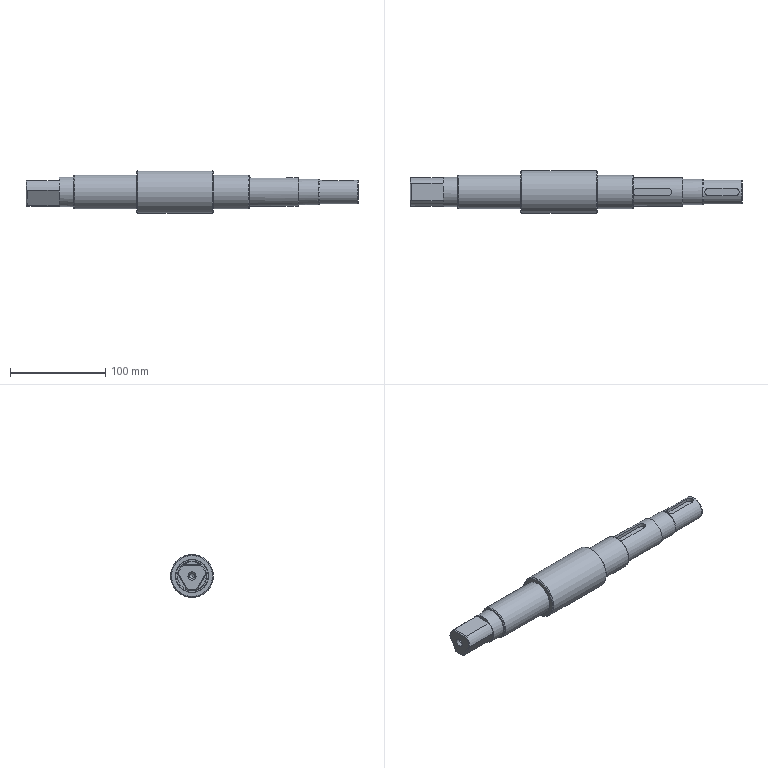NC program | NX | posted with a generic post | part box 348.4 x 45 x 45 mm
Whole program:
N10 G17 G21 G94 G90
(刀补6 , TOOL : D6)
N12 T06 M6
N14 G54
N16 G17 G0 G90 X94.077 Y-0.933 B0. C0. S4500 M3
N18 G43 Z30. H6
N20 Z-4.466
N22 G94 G1 X96.205 Z-4.578 F1000.
N24 X96.342 Y-0.932 Z-4.585
N26 X96.626 Y-0.84 Z-4.601
N28 X96.867 Y-0.664 Z-4.616
N30 X97.041 Y-0.422 Z-4.632
N32 X97.13 Y-0.137 Z-4.648
N34 Y0.137 Z-4.662
N36 X97.041 Y0.421 Z-4.678
N38 X96.867 Y0.664 Z-4.693
N40 X96.626 Y0.839 Z-4.709
N42 X96.342 Y0.931 Z-4.724
N44 X96.201 Y0.933 Z-4.732
N46 X80.298 Z-5.565
N48 G41 X80.2 Y0.95 D6
N50 X64.195 F1650.
N52 G3 X63.253 Y0. R0.95
N54 X64.195 Y-0.95 R0.95
N56 G1 X96.205
N58 G3 X97.148 Y0. R0.95
N60 X96.205 Y0.95 R0.95
N62 G1 X80.2
N64 X74.533 Z-5.664
N66 X64.195
N68 G3 X63.253 Y0. R0.95
N70 X64.195 Y-0.95 R0.95
N72 G1 X96.205
N74 G3 X97.148 Y0. R0.95
N76 X96.205 Y0.95 R0.95
N78 G1 X80.2
N80 X74.533 Z-5.763
N82 X64.195
N84 G3 X63.253 Y0. R0.95
N86 X64.195 Y-0.95 R0.95
N88 G1 X96.205
N90 G3 X97.148 Y0. R0.95
N92 X96.205 Y0.95 R0.95
N94 G1 X80.2
N96 X74.533 Z-5.862
N98 X64.195
N100 G3 X63.253 Y0. R0.95
N102 X64.195 Y-0.95 R0.95
N104 G1 X96.205
N106 G3 X97.148 Y0. R0.95
N108 X96.205 Y0.95 R0.95
N110 G1 X80.2
N112 X74.533 Z-5.961
N114 X64.195
N116 G3 X63.253 Y0. R0.95
N118 X64.195 Y-0.95 R0.95
N120 G1 X96.205
N122 G3 X97.148 Y0. R0.95
N124 X96.205 Y0.95 R0.95
N126 G1 X80.2
N128 X74.533 Z-6.06
N130 X64.195
N132 G3 X63.253 Y0. R0.95
N134 X64.195 Y-0.95 R0.95
N136 G1 X96.205
N138 G3 X97.148 Y0. R0.95
N140 X96.205 Y0.95 R0.95
N142 G1 X80.2
N144 X74.533 Z-6.159
N146 X64.195
N148 G3 X63.253 Y0. R0.95
N150 X64.195 Y-0.95 R0.95
N152 G1 X96.205
N154 G3 X97.148 Y0. R0.95
N156 X96.205 Y0.95 R0.95
N158 G1 X80.2
N160 X74.533 Z-6.258
N162 X64.195
N164 G3 X63.253 Y0. R0.95
N166 X64.195 Y-0.95 R0.95
N168 G1 X96.205
N170 G3 X97.148 Y0. R0.95
N172 X96.205 Y0.95 R0.95
N174 G1 X80.2
N176 X74.533 Z-6.357
N178 X64.195
N180 G3 X63.253 Y0. R0.95
N182 X64.195 Y-0.95 R0.95
N184 G1 X96.205
N186 G3 X97.148 Y0. R0.95
N188 X96.205 Y0.95 R0.95
N190 G1 X80.2
N192 X74.533 Z-6.455
N194 X64.195
N196 G3 X63.253 Y0. R0.95
N198 X64.195 Y-0.95 R0.95
N200 G1 X96.205
N202 G3 X97.148 Y0. R0.95
N204 X96.205 Y0.95 R0.95
N206 G1 X80.2
N208 X74.533 Z-6.554
N210 X64.195
N212 G3 X63.253 Y0. R0.95
N214 X64.195 Y-0.95 R0.95
N216 G1 X96.205
N218 G3 X97.148 Y0. R0.95
N220 X96.205 Y0.95 R0.95
N222 G1 X80.2
N224 X74.533 Z-6.653
N226 X64.195
N228 G3 X63.253 Y0. R0.95
N230 X64.195 Y-0.95 R0.95
N232 G1 X96.205
N234 G3 X97.148 Y0. R0.95
N236 X96.205 Y0.95 R0.95
N238 G1 X80.2
N240 X74.533 Z-6.752
N242 X64.195
N244 G3 X63.253 Y0. R0.95
N246 X64.195 Y-0.95 R0.95
N248 G1 X96.205
N250 G3 X97.148 Y0. R0.95
N252 X96.205 Y0.95 R0.95
N254 G1 X80.2
N256 X74.533 Z-6.851
N258 X64.195
N260 G3 X63.253 Y0. R0.95
N262 X64.195 Y-0.95 R0.95
N264 G1 X96.205
N266 G3 X97.148 Y0. R0.95
N268 X96.205 Y0.95 R0.95
N270 G1 X80.2
N272 X74.533 Z-6.95
N274 X64.195
N276 G3 X63.253 Y0. R0.95
N278 X64.195 Y-0.95 R0.95
N280 G1 X96.205
N282 G3 X97.148 Y0. R0.95
N284 X96.205 Y0.95 R0.95
N286 G1 X80.2
N288 X74.533 Z-7.049
N290 X64.195
N292 G3 X63.253 Y0. R0.95
N294 X64.195 Y-0.95 R0.95
N296 G1 X96.205
N298 G3 X97.148 Y0. R0.95
N300 X96.205 Y0.95 R0.95
N302 G1 X80.2
N304 X74.533 Z-7.148
N306 X64.195
N308 G3 X63.253 Y0. R0.95
N310 X64.195 Y-0.95 R0.95
N312 G1 X96.205
N314 G3 X97.148 Y0. R0.95
N316 X96.205 Y0.95 R0.95
N318 G1 X80.2
N320 X74.533 Z-7.247
N322 X64.195
N324 G3 X63.253 Y0. R0.95
N326 X64.195 Y-0.95 R0.95
N328 G1 X96.205
N330 G3 X97.148 Y0. R0.95
N332 X96.205 Y0.95 R0.95
N334 G1 X80.2
N336 X74.533 Z-7.346
N338 X64.195
N340 G3 X63.253 Y0. R0.95
N342 X64.195 Y-0.95 R0.95
N344 G1 X96.205
N346 G3 X97.148 Y0. R0.95
N348 X96.205 Y0.95 R0.95
N350 G1 X80.2
N352 X74.533 Z-7.445
N354 X64.195
N356 G3 X63.253 Y0. R0.95
N358 X64.195 Y-0.95 R0.95
N360 G1 X96.205
N362 G3 X97.148 Y0. R0.95
N364 X96.205 Y0.95 R0.95
N366 G1 X80.2
N368 X74.533 Z-7.543
N370 X64.2
N372 G3 X63.25 Y0. R0.95
N374 X64.2 Y-0.95 R0.95
N376 G1 X96.2
N378 G3 X97.15 Y0. R0.95
N380 X96.2 Y0.95 R0.95
N382 G1 X80.2
N384 X74.533 Z-7.642
N386 X64.2
N388 G3 X63.25 Y0. R0.95
N390 X64.2 Y-0.95 R0.95
N392 G1 X96.2
N394 G3 X97.15 Y0. R0.95
N396 X96.2 Y0.95 R0.95
N398 G1 X80.2
N400 X74.533 Z-7.741
N402 X64.2
N404 G3 X63.25 Y0. R0.95
N406 X64.2 Y-0.95 R0.95
N408 G1 X96.2
N410 G3 X97.15 Y0. R0.95
N412 X96.2 Y0.95 R0.95
N414 G1 X80.2
N416 X74.533 Z-7.84
N418 X64.2
N420 G3 X63.25 Y0. R0.95
N422 X64.2 Y-0.95 R0.95
N424 G1 X96.2
N426 G3 X97.15 Y0. R0.95
N428 X96.2 Y0.95 R0.95
N430 G1 X80.2
N432 X74.533 Z-7.939
N434 X64.2
N436 G3 X63.25 Y0. R0.95
N438 X64.2 Y-0.95 R0.95
N440 G1 X96.2
N442 G3 X97.15 Y0. R0.95
N444 X96.2 Y0.95 R0.95
N446 G1 X80.2
N448 X74.533 Z-8.038
N450 X64.2
N452 G3 X63.25 Y0. R0.95
N454 X64.2 Y-0.95 R0.95
N456 G1 X96.2
N458 G3 X97.15 Y0. R0.95
N460 X96.2 Y0.95 R0.95
N462 G1 X80.2
N464 X74.533 Z-8.137
N466 X64.2
N468 G3 X63.25 Y0. R0.95
N470 X64.2 Y-0.95 R0.95
N472 G1 X96.2
N474 G3 X97.15 Y0. R0.95
N476 X96.2 Y0.95 R0.95
N478 G1 X80.2
N480 X74.533 Z-8.236
N482 X64.2
N484 G3 X63.25 Y0. R0.95
N486 X64.2 Y-0.95 R0.95
N488 G1 X96.2
N490 G3 X97.15 Y0. R0.95
N492 X96.2 Y0.95 R0.95
N494 G1 X80.2
N496 X74.533 Z-8.335
N498 X64.2
N500 G3 X63.25 Y0. R0.95
N502 X64.2 Y-0.95 R0.95
N504 G1 X96.2
N506 G3 X97.15 Y0. R0.95
N508 X96.2 Y0.95 R0.95
N510 G1 X80.2
N512 X74.533 Z-8.434
N514 X64.2
N516 G3 X63.25 Y0. R0.95
N518 X64.2 Y-0.95 R0.95
N520 G1 X96.2
N522 G3 X97.15 Y0. R0.95
N524 X96.2 Y0.95 R0.95
N526 G1 X80.2
N528 X74.533 Z-8.533
N530 X64.2
N532 G3 X63.25 Y0. R0.95
N534 X64.2 Y-0.95 R0.95
N536 G1 X96.2
N538 G3 X97.15 Y0. R0.95
N540 X96.2 Y0.95 R0.95
N542 G1 X80.2
N544 X74.533 Z-8.632
N546 X64.2
N548 G3 X63.25 Y0. R0.95
N550 X64.2 Y-0.95 R0.95
N552 G1 X96.2
N554 G3 X97.15 Y0. R0.95
N556 X96.2 Y0.95 R0.95
N558 G1 X80.2
N560 X74.533 Z-8.73
N562 X64.2
N564 G3 X63.25 Y0. R0.95
N566 X64.2 Y-0.95 R0.95
N568 G1 X96.2
N570 G3 X97.15 Y0. R0.95
N572 X96.2 Y0.95 R0.95
N574 G1 X80.2
N576 X74.533 Z-8.829
N578 X64.2
N580 G3 X63.25 Y0. R0.95
N582 X64.2 Y-0.95 R0.95
N584 G1 X96.2
N586 G3 X97.15 Y0. R0.95
N588 X96.2 Y0.95 R0.95
N590 G1 X80.2
N592 X74.533 Z-8.928
N594 X64.2
N596 G3 X63.25 Y0. R0.95
N598 X64.2 Y-0.95 R0.95
N600 G1 X96.2
N602 G3 X97.15 Y0. R0.95
N604 X96.2 Y0.95 R0.95
N606 G1 X80.2
N608 X74.533 Z-9.027
N610 X64.2
N612 G3 X63.25 Y0. R0.95
N614 X64.2 Y-0.95 R0.95
N616 G1 X96.2
N618 G3 X97.15 Y0. R0.95
N620 X96.2 Y0.95 R0.95
N622 G1 X80.2
N624 X74.533 Z-9.126
N626 X64.2
N628 G3 X63.25 Y0. R0.95
N630 X64.2 Y-0.95 R0.95
N632 G1 X96.2
N634 G3 X97.15 Y0. R0.95
N636 X96.2 Y0.95 R0.95
N638 G1 X80.2
N640 X74.533 Z-9.225
N642 X64.2
N644 G3 X63.25 Y0. R0.95
N646 X64.2 Y-0.95 R0.95
N648 G1 X96.2
N650 G3 X97.15 Y0. R0.95
N652 X96.2 Y0.95 R0.95
N654 G1 X80.2
N656 X74.533 Z-9.324
N658 X64.2
N660 G3 X63.25 Y0. R0.95
N662 X64.2 Y-0.95 R0.95
N664 G1 X96.2
N666 G3 X97.15 Y0. R0.95
N668 X96.2 Y0.95 R0.95
N670 G1 X80.2
N672 X74.533 Z-9.423
N674 X64.2
N676 G3 X63.25 Y0. R0.95
N678 X64.2 Y-0.95 R0.95
N680 G1 X96.2
N682 G3 X97.15 Y0. R0.95
N684 X96.2 Y0.95 R0.95
N686 G1 X80.2
N688 X74.533 Z-9.522
N690 X64.2
N692 G3 X63.25 Y0. R0.95
N694 X64.2 Y-0.95 R0.95
N696 G1 X96.2
N698 G3 X97.15 Y0. R0.95
N700 X96.2 Y0.95 R0.95
N702 G1 X80.2
N704 X74.533 Z-9.621
N706 X64.2
N708 G3 X63.25 Y0. R0.95
N710 X64.2 Y-0.95 R0.95
N712 G1 X96.2
N714 G3 X97.15 Y0. R0.95
N716 X96.2 Y0.95 R0.95
N718 G1 X80.2
N720 X74.533 Z-9.72
N722 X64.2
N724 G3 X63.25 Y0. R0.95
N726 X64.2 Y-0.95 R0.95
N728 G1 X96.2
N730 G3 X97.15 Y0. R0.95
N732 X96.2 Y0.95 R0.95
N734 G1 X80.2
N736 X74.533 Z-9.818
N738 X64.2
N740 G3 X63.25 Y0. R0.95
N742 X64.2 Y-0.95 R0.95
N744 G1 X96.2
N746 G3 X97.15 Y0. R0.95
N748 X96.2 Y0.95 R0.95
N750 G1 X80.2
N752 X74.533 Z-9.917
N754 X64.2
N756 G3 X63.25 Y0. R0.95
N758 X64.2 Y-0.95 R0.95
N760 G1 X96.2
N762 G3 X97.15 Y0. R0.95
N764 X96.2 Y0.95 R0.95
N766 G1 X80.2
N768 X74.533 Z-10.016
N770 X64.2
N772 G3 X63.25 Y0. R0.95
N774 X64.2 Y-0.95 R0.95
N776 G1 X96.2
N778 G3 X97.15 Y0. R0.95
N780 X96.2 Y0.95 R0.95
N782 G1 X80.2
N784 X74.533 Z-10.115
N786 X64.2
N788 G3 X63.25 Y0. R0.95
N790 X64.2 Y-0.95 R0.95
N792 G1 X96.2
N794 G3 X97.15 Y0. R0.95
N796 X96.2 Y0.95 R0.95
N798 G1 X80.2
N800 X74.533 Z-10.214
N802 X64.2
N804 G3 X63.25 Y0. R0.95
N806 X64.2 Y-0.95 R0.95
N808 G1 X96.2
N810 G3 X97.15 Y0. R0.95
N812 X96.2 Y0.95 R0.95
N814 G1 X80.2
N816 X74.533 Z-10.313
N818 X64.2
N820 G3 X63.25 Y0. R0.95
N822 X64.2 Y-0.95 R0.95
N824 G1 X96.2
N826 G3 X97.15 Y0. R0.95
N828 X96.2 Y0.95 R0.95
N830 G1 X80.2
N832 X74.533 Z-10.412
N834 X64.2
N836 G3 X63.25 Y0. R0.95
N838 X64.2 Y-0.95 R0.95
N840 G1 X96.2
N842 G3 X97.15 Y0. R0.95
N844 X96.2 Y0.95 R0.95
N846 G1 X80.2
N848 X74.533 Z-10.511
N850 X64.2
N852 G3 X63.25 Y0. R0.95
N854 X64.2 Y-0.95 R0.95
N856 G1 X96.2
N858 G3 X97.15 Y0. R0.95
N860 X96.2 Y0.95 R0.95
N862 G1 X80.2
N864 X74.533 Z-10.61
N866 X64.2
N868 G3 X63.25 Y0. R0.95
N870 X64.2 Y-0.95 R0.95
N872 G1 X96.2
N874 G3 X97.15 Y0. R0.95
N876 X96.2 Y0.95 R0.95
N878 G1 X80.2
N880 X74.533 Z-10.709
N882 X64.2
N884 G3 X63.25 Y0. R0.95
N886 X64.2 Y-0.95 R0.95
N888 G1 X96.2
N890 G3 X97.15 Y0. R0.95
N892 X96.2 Y0.95 R0.95
N894 G1 X80.2
N896 X74.533 Z-10.808
N898 X64.2
N900 G3 X63.25 Y0. R0.95
N902 X64.2 Y-0.95 R0.95
N904 G1 X96.2
N906 G3 X97.15 Y0. R0.95
N908 X96.2 Y0.95 R0.95
N910 G1 X80.2
N912 X74.533 Z-10.907
N914 X64.2
N916 G3 X63.25 Y0. R0.95
N918 X64.2 Y-0.95 R0.95
N920 G1 X96.2
N922 G3 X97.15 Y0. R0.95
N924 X96.2 Y0.95 R0.95
N926 G1 X80.2
N928 X74.533 Z-11.005
N930 X64.2
N932 G3 X63.25 Y0. R0.95
N934 X64.2 Y-0.95 R0.95
N936 G1 X96.2
N938 G3 X97.15 Y0. R0.95
N940 X96.2 Y0.95 R0.95
N942 G1 X80.2
N944 X74.533 Z-11.104
N946 X64.2
N948 G3 X63.25 Y0. R0.95
N950 X64.2 Y-0.95 R0.95
N952 G1 X96.2
N954 G3 X97.15 Y0. R0.95
N956 X96.2 Y0.95 R0.95
N958 G1 X80.2
N960 X74.533 Z-11.203
N962 X64.2
N964 G3 X63.25 Y0. R0.95
N966 X64.2 Y-0.95 R0.95
N968 G1 X96.2
N970 G3 X97.15 Y0. R0.95
N972 X96.2 Y0.95 R0.95
N974 G1 X80.2
N976 X74.533 Z-11.302
N978 X64.2
N980 G3 X63.25 Y0. R0.95
N982 X64.2 Y-0.95 R0.95
N984 G1 X96.2
N986 G3 X97.15 Y0. R0.95
N988 X96.2 Y0.95 R0.95
N990 G1 X80.2
N992 X74.533 Z-11.401
N994 X64.2
N996 G3 X63.25 Y0. R0.95
N998 X64.2 Y-0.95 R0.95
N1000 G1 X96.2
N1002 G3 X97.15 Y0. R0.95
N1004 X96.2 Y0.95 R0.95
N1006 G1 X80.2
N1008 X74.533 Z-11.5
N1010 X64.2
N1012 G3 X63.25 Y0. R0.95
N1014 X64.2 Y-0.95 R0.95
N1016 G1 X96.2
N1018 G3 X97.15 Y0. R0.95
N1020 X96.2 Y0.95 R0.95
N1022 G1 X74.533
N1024 G40
N1026 X74.435 Y0.933
N1028 Z-10.5
N1030 G0 Z30.
(刀补6_COPY , TOOL : D6)
N1032 X163.085 Y-0.933
N1034 Z-8.466
N1036 G1 X167.206 Z-8.682 F1000.
N1038 X167.343 Y-0.932 Z-8.689
N1040 X167.627 Y-0.84 Z-8.705
N1042 X167.867 Y-0.664 Z-8.721
N1044 X168.041 Y-0.422 Z-8.736
N1046 X168.131 Y-0.137 Z-8.752
N1048 Y0.137 Z-8.766
N1050 X168.041 Y0.421 Z-8.782
N1052 X167.867 Y0.663 Z-8.798
N1054 X167.627 Y0.839 Z-8.813
N1056 X167.343 Y0.931 Z-8.829
N1058 X167.202 Y0.933 Z-8.836
N1060 X153.298 Z-9.565
N1062 G41 X153.2 Y0.95
N1064 X139.194 F1650.
N1066 G3 X138.252 Y0. R0.95
N1068 X139.194 Y-0.95 R0.95
N1070 G1 X167.206
N1072 G3 X168.148 Y0. R0.95
N1074 X167.206 Y0.95 R0.95
N1076 G1 X153.2
N1078 X147.554 Z-9.663
N1080 X139.194
N1082 G3 X138.252 Y0. R0.95
N1084 X139.194 Y-0.95 R0.95
N1086 G1 X167.206
N1088 G3 X168.148 Y0. R0.95
N1090 X167.206 Y0.95 R0.95
N1092 G1 X153.2
N1094 X147.554 Z-9.762
N1096 X139.194
N1098 G3 X138.252 Y0. R0.95
N1100 X139.194 Y-0.95 R0.95
N1102 G1 X167.206
N1104 G3 X168.148 Y0. R0.95
N1106 X167.206 Y0.95 R0.95
N1108 G1 X153.2
N1110 X147.554 Z-9.861
N1112 X139.194
N1114 G3 X138.252 Y0. R0.95
N1116 X139.194 Y-0.95 R0.95
N1118 G1 X167.206
N1120 G3 X168.148 Y0. R0.95
N1122 X167.206 Y0.95 R0.95
N1124 G1 X153.2
N1126 X147.554 Z-9.959
N1128 X139.194
N1130 G3 X138.252 Y0. R0.95
N1132 X139.194 Y-0.95 R0.95
N1134 G1 X167.206
N1136 G3 X168.148 Y0. R0.95
N1138 X167.206 Y0.95 R0.95
N1140 G1 X153.2
N1142 X147.554 Z-10.058
N1144 X139.2
N1146 G3 X138.25 Y0. R0.95
N1148 X139.2 Y-0.95 R0.95
N1150 G1 X167.2
N1152 G3 X168.15 Y0. R0.95
N1154 X167.2 Y0.95 R0.95
N1156 G1 X153.2
N1158 X147.554 Z-10.156
N1160 X139.2
N1162 G3 X138.25 Y0. R0.95
N1164 X139.2 Y-0.95 R0.95
N1166 G1 X167.2
N1168 G3 X168.15 Y0. R0.95
N1170 X167.2 Y0.95 R0.95
N1172 G1 X153.2
N1174 X147.554 Z-10.255
N1176 X139.2
N1178 G3 X138.25 Y0. R0.95
N1180 X139.2 Y-0.95 R0.95
N1182 G1 X167.2
N1184 G3 X168.15 Y0. R0.95
N1186 X167.2 Y0.95 R0.95
N1188 G1 X153.2
N1190 X147.554 Z-10.353
N1192 X139.2
N1194 G3 X138.25 Y0. R0.95
N1196 X139.2 Y-0.95 R0.95
N1198 G1 X167.2
N1200 G3 X168.15 Y0. R0.95
N1202 X167.2 Y0.95 R0.95
N1204 G1 X153.2
N1206 X147.554 Z-10.452
N1208 X139.2
N1210 G3 X138.25 Y0. R0.95
N1212 X139.2 Y-0.95 R0.95
N1214 G1 X167.2
N1216 G3 X168.15 Y0. R0.95
N1218 X167.2 Y0.95 R0.95
N1220 G1 X153.2
N1222 X147.554 Z-10.55
N1224 X139.2
N1226 G3 X138.25 Y0. R0.95
N1228 X139.2 Y-0.95 R0.95
N1230 G1 X167.2
N1232 G3 X168.15 Y0. R0.95
N1234 X167.2 Y0.95 R0.95
N1236 G1 X153.2
N1238 X147.554 Z-10.649
N1240 X139.2
N1242 G3 X138.25 Y0. R0.95
N1244 X139.2 Y-0.95 R0.95
N1246 G1 X167.2
N1248 G3 X168.15 Y0. R0.95
N1250 X167.2 Y0.95 R0.95
N1252 G1 X153.2
N1254 X147.554 Z-10.748
N1256 X139.2
N1258 G3 X138.25 Y0. R0.95
N1260 X139.2 Y-0.95 R0.95
N1262 G1 X167.2
N1264 G3 X168.15 Y0. R0.95
N1266 X167.2 Y0.95 R0.95
N1268 G1 X153.2
N1270 X147.554 Z-10.846
N1272 X139.2
N1274 G3 X138.25 Y0. R0.95
N1276 X139.2 Y-0.95 R0.95
N1278 G1 X167.2
N1280 G3 X168.15 Y0. R0.95
N1282 X167.2 Y0.95 R0.95
N1284 G1 X153.2
N1286 X147.554 Z-10.945
N1288 X139.2
N1290 G3 X138.25 Y0. R0.95
N1292 X139.2 Y-0.95 R0.95
N1294 G1 X167.2
N1296 G3 X168.15 Y0. R0.95
N1298 X167.2 Y0.95 R0.95
N1300 G1 X153.2
N1302 X147.554 Z-11.043
N1304 X139.2
N1306 G3 X138.25 Y0. R0.95
N1308 X139.2 Y-0.95 R0.95
N1310 G1 X167.2
N1312 G3 X168.15 Y0. R0.95
N1314 X167.2 Y0.95 R0.95
N1316 G1 X153.2
N1318 X147.554 Z-11.142
N1320 X139.2
N1322 G3 X138.25 Y0. R0.95
N1324 X139.2 Y-0.95 R0.95
N1326 G1 X167.2
N1328 G3 X168.15 Y0. R0.95
N1330 X167.2 Y0.95 R0.95
N1332 G1 X153.2
N1334 X147.554 Z-11.24
N1336 X139.2
N1338 G3 X138.25 Y0. R0.95
N1340 X139.2 Y-0.95 R0.95
N1342 G1 X167.2
N1344 G3 X168.15 Y0. R0.95
N1346 X167.2 Y0.95 R0.95
N1348 G1 X153.2
N1350 X147.554 Z-11.339
N1352 X139.2
N1354 G3 X138.25 Y0. R0.95
N1356 X139.2 Y-0.95 R0.95
N1358 G1 X167.2
N1360 G3 X168.15 Y0. R0.95
N1362 X167.2 Y0.95 R0.95
N1364 G1 X153.2
N1366 X147.554 Z-11.437
N1368 X139.2
N1370 G3 X138.25 Y0. R0.95
N1372 X139.2 Y-0.95 R0.95
N1374 G1 X167.2
N1376 G3 X168.15 Y0. R0.95
N1378 X167.2 Y0.95 R0.95
N1380 G1 X153.2
N1382 X147.554 Z-11.536
N1384 X139.2
N1386 G3 X138.25 Y0. R0.95
N1388 X139.2 Y-0.95 R0.95
N1390 G1 X167.2
N1392 G3 X168.15 Y0. R0.95
N1394 X167.2 Y0.95 R0.95
N1396 G1 X153.2
N1398 X147.554 Z-11.635
N1400 X139.2
N1402 G3 X138.25 Y0. R0.95
N1404 X139.2 Y-0.95 R0.95
N1406 G1 X167.2
N1408 G3 X168.15 Y0. R0.95
N1410 X167.2 Y0.95 R0.95
N1412 G1 X153.2
N1414 X147.554 Z-11.733
N1416 X139.2
N1418 G3 X138.25 Y0. R0.95
N1420 X139.2 Y-0.95 R0.95
N1422 G1 X167.2
N1424 G3 X168.15 Y0. R0.95
N1426 X167.2 Y0.95 R0.95
N1428 G1 X153.2
N1430 X147.554 Z-11.832
N1432 X139.2
N1434 G3 X138.25 Y0. R0.95
N1436 X139.2 Y-0.95 R0.95
N1438 G1 X167.2
N1440 G3 X168.15 Y0. R0.95
N1442 X167.2 Y0.95 R0.95
N1444 G1 X153.2
N1446 X147.554 Z-11.93
N1448 X139.2
N1450 G3 X138.25 Y0. R0.95
N1452 X139.2 Y-0.95 R0.95
N1454 G1 X167.2
N1456 G3 X168.15 Y0. R0.95
N1458 X167.2 Y0.95 R0.95
N1460 G1 X153.2
N1462 X147.554 Z-12.029
N1464 X139.2
N1466 G3 X138.25 Y0. R0.95
N1468 X139.2 Y-0.95 R0.95
N1470 G1 X167.2
N1472 G3 X168.15 Y0. R0.95
N1474 X167.2 Y0.95 R0.95
N1476 G1 X153.2
N1478 X147.554 Z-12.127
N1480 X139.2
N1482 G3 X138.25 Y0. R0.95
N1484 X139.2 Y-0.95 R0.95
N1486 G1 X167.2
N1488 G3 X168.15 Y0. R0.95
N1490 X167.2 Y0.95 R0.95
N1492 G1 X153.2
N1494 X147.554 Z-12.226
N1496 X139.2
N1498 G3 X138.25 Y0. R0.95
N1500 X139.2 Y-0.95 R0.95
N1502 G1 X167.2
N1504 G3 X168.15 Y0. R0.95
N1506 X167.2 Y0.95 R0.95
N1508 G1 X153.2
N1510 X147.554 Z-12.325
N1512 X139.2
N1514 G3 X138.25 Y0. R0.95
N1516 X139.2 Y-0.95 R0.95
N1518 G1 X167.2
N1520 G3 X168.15 Y0. R0.95
N1522 X167.2 Y0.95 R0.95
N1524 G1 X153.2
N1526 X147.554 Z-12.423
N1528 X139.2
N1530 G3 X138.25 Y0. R0.95
N1532 X139.2 Y-0.95 R0.95
N1534 G1 X167.2
N1536 G3 X168.15 Y0. R0.95
N1538 X167.2 Y0.95 R0.95
N1540 G1 X153.2
N1542 X147.554 Z-12.522
N1544 X139.2
N1546 G3 X138.25 Y0. R0.95
N1548 X139.2 Y-0.95 R0.95
N1550 G1 X167.2
N1552 G3 X168.15 Y0. R0.95
N1554 X167.2 Y0.95 R0.95
N1556 G1 X153.2
N1558 X147.554 Z-12.62
N1560 X139.2
N1562 G3 X138.25 Y0. R0.95
N1564 X139.2 Y-0.95 R0.95
N1566 G1 X167.2
N1568 G3 X168.15 Y0. R0.95
N1570 X167.2 Y0.95 R0.95
N1572 G1 X153.2
N1574 X147.554 Z-12.719
N1576 X139.2
N1578 G3 X138.25 Y0. R0.95
N1580 X139.2 Y-0.95 R0.95
N1582 G1 X167.2
N1584 G3 X168.15 Y0. R0.95
N1586 X167.2 Y0.95 R0.95
N1588 G1 X153.2
N1590 X147.554 Z-12.817
N1592 X139.2
N1594 G3 X138.25 Y0. R0.95
N1596 X139.2 Y-0.95 R0.95
N1598 G1 X167.2
N1600 G3 X168.15 Y0. R0.95
N1602 X167.2 Y0.95 R0.95
N1604 G1 X153.2
N1606 X147.554 Z-12.916
N1608 X139.2
N1610 G3 X138.25 Y0. R0.95
N1612 X139.2 Y-0.95 R0.95
N1614 G1 X167.2
N1616 G3 X168.15 Y0. R0.95
N1618 X167.2 Y0.95 R0.95
N1620 G1 X153.2
N1622 X147.554 Z-13.014
N1624 X139.2
N1626 G3 X138.25 Y0. R0.95
N1628 X139.2 Y-0.95 R0.95
N1630 G1 X167.2
N1632 G3 X168.15 Y0. R0.95
N1634 X167.2 Y0.95 R0.95
N1636 G1 X153.2
N1638 X147.554 Z-13.113
N1640 X139.2
N1642 G3 X138.25 Y0. R0.95
N1644 X139.2 Y-0.95 R0.95
N1646 G1 X167.2
N1648 G3 X168.15 Y0. R0.95
N1650 X167.2 Y0.95 R0.95
N1652 G1 X153.2
N1654 X147.554 Z-13.212
N1656 X139.2
N1658 G3 X138.25 Y0. R0.95
N1660 X139.2 Y-0.95 R0.95
N1662 G1 X167.2
N1664 G3 X168.15 Y0. R0.95
N1666 X167.2 Y0.95 R0.95
N1668 G1 X153.2
N1670 X147.554 Z-13.31
N1672 X139.2
N1674 G3 X138.25 Y0. R0.95
N1676 X139.2 Y-0.95 R0.95
N1678 G1 X167.2
N1680 G3 X168.15 Y0. R0.95
N1682 X167.2 Y0.95 R0.95
N1684 G1 X153.2
N1686 X147.554 Z-13.409
N1688 X139.2
N1690 G3 X138.25 Y0. R0.95
N1692 X139.2 Y-0.95 R0.95
N1694 G1 X167.2
N1696 G3 X168.15 Y0. R0.95
N1698 X167.2 Y0.95 R0.95
N1700 G1 X153.2
N1702 X147.554 Z-13.507
N1704 X139.2
N1706 G3 X138.25 Y0. R0.95
N1708 X139.2 Y-0.95 R0.95
N1710 G1 X167.2
N1712 G3 X168.15 Y0. R0.95
N1714 X167.2 Y0.95 R0.95
N1716 G1 X153.2
N1718 X147.554 Z-13.606
N1720 X139.2
N1722 G3 X138.25 Y0. R0.95
N1724 X139.2 Y-0.95 R0.95
N1726 G1 X167.2
N1728 G3 X168.15 Y0. R0.95
N1730 X167.2 Y0.95 R0.95
N1732 G1 X153.2
N1734 X147.554 Z-13.704
N1736 X139.2
N1738 G3 X138.25 Y0. R0.95
N1740 X139.2 Y-0.95 R0.95
N1742 G1 X167.2
N1744 G3 X168.15 Y0. R0.95
N1746 X167.2 Y0.95 R0.95
N1748 G1 X153.2
N1750 X147.554 Z-13.803
N1752 X139.2
N1754 G3 X138.25 Y0. R0.95
N1756 X139.2 Y-0.95 R0.95
N1758 G1 X167.2
N1760 G3 X168.15 Y0. R0.95
N1762 X167.2 Y0.95 R0.95
N1764 G1 X153.2
N1766 X147.554 Z-13.901
N1768 X139.2
N1770 G3 X138.25 Y0. R0.95
N1772 X139.2 Y-0.95 R0.95
N1774 G1 X167.2
N1776 G3 X168.15 Y0. R0.95
N1778 X167.2 Y0.95 R0.95
N1780 G1 X153.2
N1782 X147.554 Z-14.
N1784 X139.2
N1786 G3 X138.25 Y0. R0.95
N1788 X139.2 Y-0.95 R0.95
N1790 G1 X167.2
N1792 G3 X168.15 Y0. R0.95
N1794 X167.2 Y0.95 R0.95
N1796 G1 X147.554
N1798 G40
N1800 X147.455 Y0.933
N1802 Z-13.
N1804 G0 Z30.
N1806 M5
N1808 M2